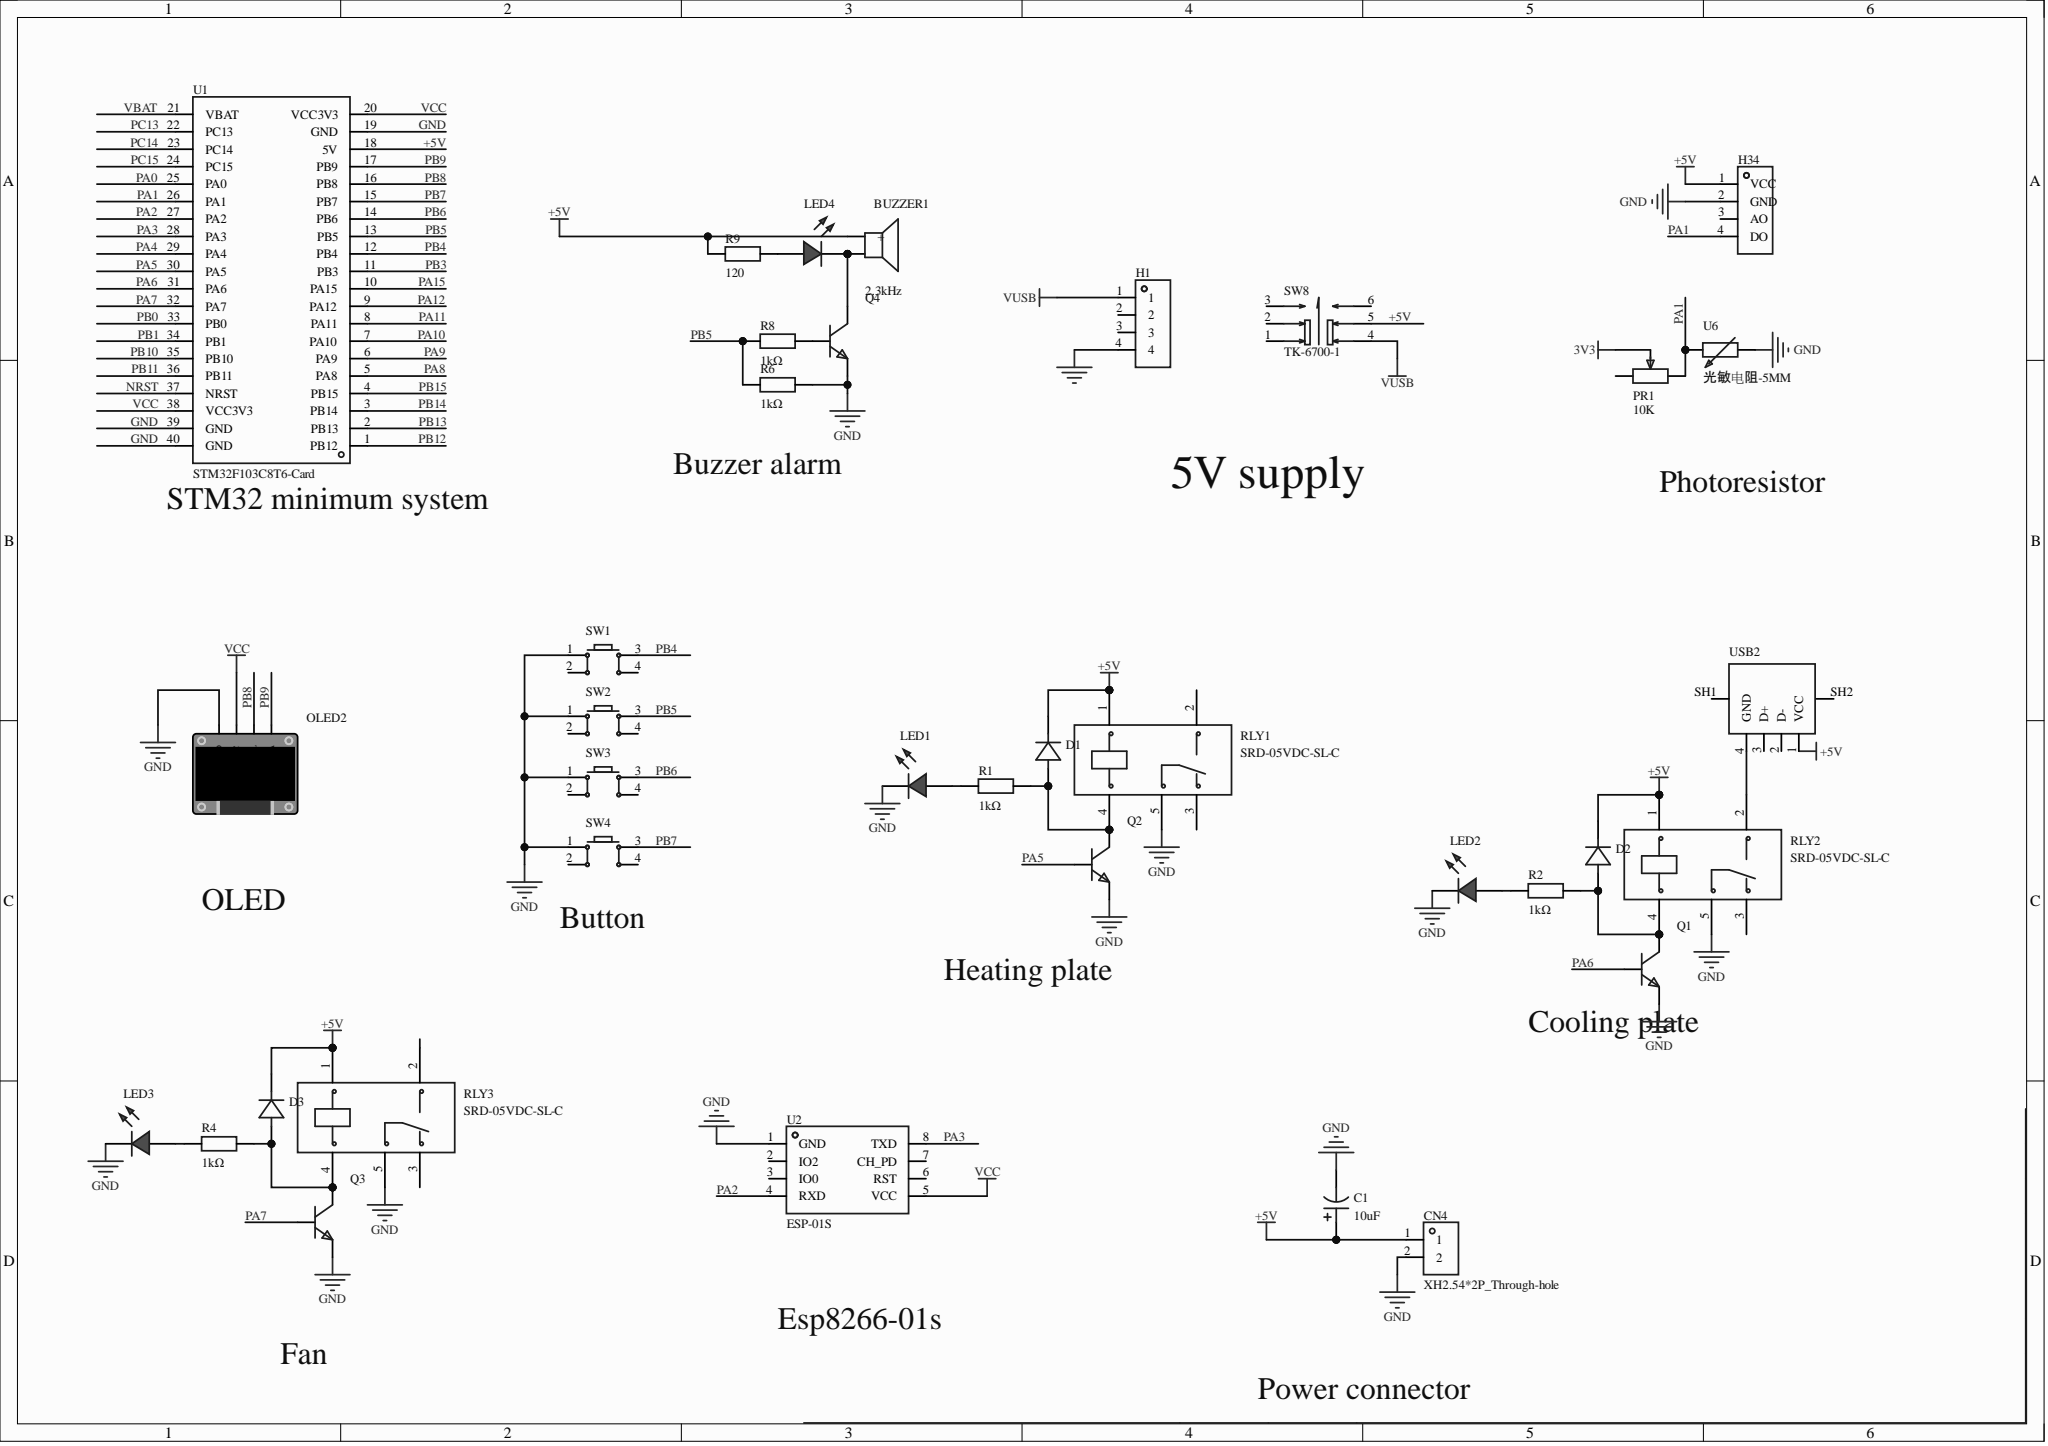Circuit board | Altium Designer | 36 parts | 26 nets
Bill of materials:
Comment,Description,Designator,Footprint,LibRef,Quantity
"2.3kHz","Drive mode:Active (built-in driver circuit);Construction type:Electromagnetic;Rated voltage:5V;Frequency:2.3kHz;Sound pressure (SPL):85dB@5V,10cm;","BUZZER1","BUZ-TH_BD12.0-P7.60-D0.6-FD","TMB12A05_C96093","1"
"10uF","Capacitance:10uF;Tolerance:±20%;Rated voltage:50V;Ripple current:120mA@100KHz;Equivalent series resistance (ESR):1.6Ω;","C1","CAP-TH_BD5.0-P2.00-D0.8-FD-10UF50VC110GL","10UF50VC110GL","1"
"XH2.54*2P_Through-hole","","CN4","CONN-TH_2P-P2.50-XH2.54-2P","XH2.54*2P_直插","1"
"","","D1, D2, D3","DO_1N4007","D_1N4007A","3"
"","","H1, H34","HDR-TH_4P-P2.54-V-F","HDR-F_2.54_1x4P","2"
"","","LED1, LED2, LED3, LED4","LED_TH-3mm","LED_TH-R_3mm","4"
"","","OLED2","0.96OLED_4P","0.96OLED模块_4P","1"
"10K","","PR1","R_3386P","R_3386P","1"
"","","Q1, Q2, Q3, Q4","S8050_TO_92","S8050_TO_NPN","4"
"1kΩ","","R1, R2, R4, R6, R8","Res_1/4W","Res_AXIAL-1/8W, Res_AXIAL-1/4W","5"
"120","","R9","Res_1/4W","Res_AXIAL-1/4W","1"
"SRD-05VDC-SL-C","","RLY1, RLY2, RLY3","RELAY-TH_SRD-XXVDC-XL-C","SRD-05VDC-SL-C","3"
"","","SW1, SW2, SW3, SW4","SW-TH_4P-L6.0-W6.0-P4.50-LS6.5","Key_TH_6x6x6","4"
"TK-6700-1","","SW8","SW-TH_TK-6700-1","TK-6700-1","1"
"STM32F103C8T6-Card","","U1","CONN-TH_L53.3-W22.9_STM32F103C8T6-CARD","STM32F103C8T6-Card","1"
"ESP-01S","","U2","WIFIM-TH_ESP-01S","ESP-01S_C111009","1"
"光敏电阻-5MM","","U6","RES-TH_L4.9-W4.3-P3.4","光敏电阻-5MM","1"
"","","USB2","USB_ Type-A","USB_ Type-A","1"
Netlist (Protel format):
[
BUZZER1
BUZ-TH_BD12.0-P7.60-D0.6-FD
2.3kHz



]
[
C1
CAP-TH_BD5.0-P2.00-D0.8-FD-10UF50VC110GL
10uF



]
[
CN4
CONN-TH_2P-P2.50-XH2.54-2P
XH2.54*2P_Through-hole



]
[
D1
DO_1N4007




]
[
D2
DO_1N4007




]
[
D3
DO_1N4007




]
[
H1
HDR-TH_4P-P2.54-V-F




]
[
H34
HDR-TH_4P-P2.54-V-F




]
[
LED1
LED_TH-3mm




]
[
LED2
LED_TH-3mm




]
[
LED3
LED_TH-3mm




]
[
LED4
LED_TH-3mm




]
[
OLED2
0.96OLED_4P




]
[
PR1
R_3386P
10K



]
[
Q1
S8050_TO_92




]
[
Q2
S8050_TO_92




]
[
Q3
S8050_TO_92




]
[
Q4
S8050_TO_92




]
[
R1
Res_1/4W
1kΩ



]
[
R2
Res_1/4W
1kΩ



]
[
R4
Res_1/4W
1kΩ



]
[
R6
Res_1/4W
1kΩ



]
[
R8
Res_1/4W
1kΩ



]
[
R9
Res_1/4W
120



]
[
RLY1
RELAY-TH_SRD-XXVDC-XL-C
SRD-05VDC-SL-C



]
[
RLY2
RELAY-TH_SRD-XXVDC-XL-C
SRD-05VDC-SL-C



]
[
RLY3
RELAY-TH_SRD-XXVDC-XL-C
SRD-05VDC-SL-C



]
[
SW1
SW-TH_4P-L6.0-W6.0-P4.50-LS6.5




]
[
SW2
SW-TH_4P-L6.0-W6.0-P4.50-LS6.5




]
[
SW3
SW-TH_4P-L6.0-W6.0-P4.50-LS6.5




]
[
SW4
SW-TH_4P-L6.0-W6.0-P4.50-LS6.5




]
[
SW8
SW-TH_TK-6700-1
TK-6700-1



]
[
U1
CONN-TH_L53.3-W22.9_STM32F103C8T6-CARD
STM32F103C8T6-Card



]
[
U2
WIFIM-TH_ESP-01S
ESP-01S



]
[
U6
RES-TH_L4.9-W4.3-P3.4
光敏电阻-5MM



]
[
USB2
USB_ Type-A




]
(
VUSB
H1-1
SW8-4
)
(
VCC
OLED2-2
U1-20
U1-38
U2-5
)
(
PB9
OLED2-4
U1-17
)
(
PB8
OLED2-3
U1-16
)
(
PB7
SW4-3
U1-15
)
(
PB6
SW3-3
U1-14
)
(
PB5
R6-1
R8-1
SW2-3
U1-13
)
(
PB4
SW1-3
U1-12
)
(
PA7
Q3-2
U1-32
)
(
PA6
Q1-2
U1-31
)
(
PA5
Q2-2
U1-30
)
(
PA3
U1-28
U2-8
)
(
PA2
U1-27
U2-4
)
(
PA1
H34-4
PR1-1
U1-26
U6-2
)
(
NetRLY2_2
RLY2-2
USB2-4
)
(
NetQ4_2
Q4-2
R8-2
)
(
NetLED4_1
LED4-1
R9-2
)
(
NetLED3_1
LED3-1
R4-1
)
(
NetLED2_1
LED2-1
R2-1
)
(
NetLED1_1
LED1-1
R1-1
)
(
NetD3_2
D3-2
Q3-3
R4-2
RLY3-4
)
(
NetD2_2
D2-2
Q1-3
R2-2
RLY2-4
)
(
NetD1_2
D1-2
Q2-3
R1-2
RLY1-4
)
(
NetBUZZER1_2
BUZZER1-2
LED4-2
Q4-3
)
(
GND
C1-2
CN4-2
H1-4
H34-2
LED1-2
LED2-2
LED3-2
OLED2-1
Q1-1
Q2-1
Q3-1
Q4-1
R6-2
RLY1-5
RLY2-5
RLY3-5
SW1-1
SW2-1
SW3-1
SW4-1
U1-19
U1-39
U1-40
U2-1
U6-1
)
(
+5V
BUZZER1-1
C1-1
CN4-1
D1-1
D2-1
D3-1
H34-1
R9-1
RLY1-1
RLY2-1
RLY3-1
SW8-5
U1-18
USB2-1
)